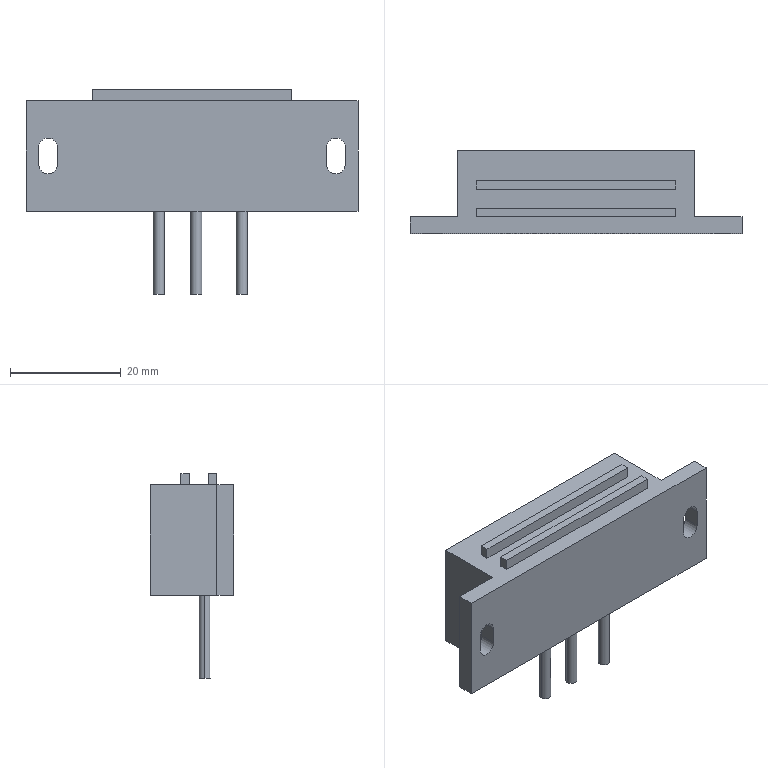Part | STEP file | magnetic latch HGE11-52-L150 | 1 solid | 39 faces | box 60 x 15 x 37 mm | volume 14160 mm3 | plane 27 | cylinder 12 | commonest cylinder face diameters 2 x6 3.4 x6